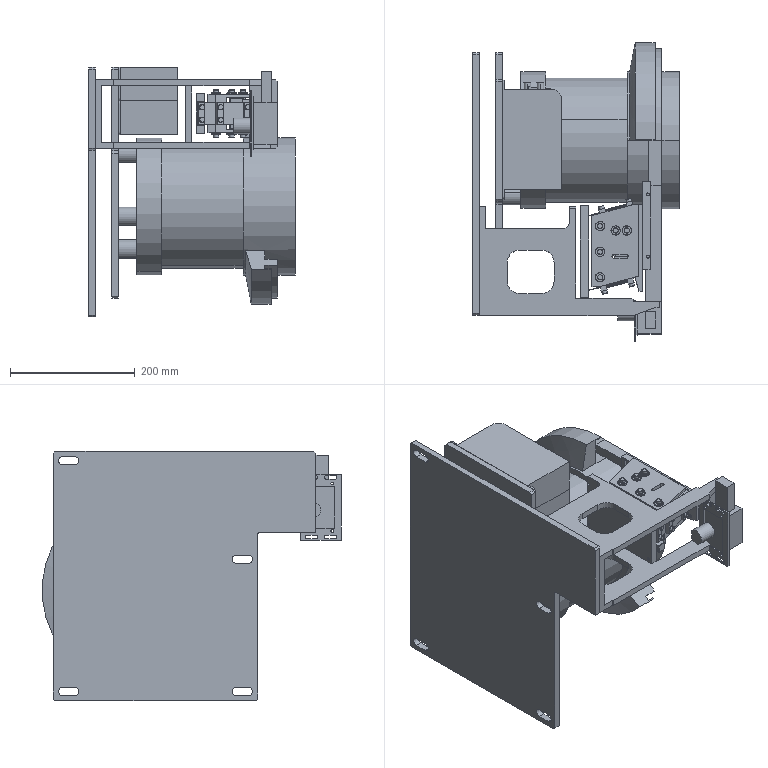Part | STEP file | COMPANY_C blow-air scheme, small part | 14 solids | 1107 faces | box 330.519 x 479.611 x 400.249 mm | volume 15256287 mm3 | plane 618 | cylinder 396 | spline 92 | cone 1 | commonest cylinder face diameters 4.3 x66 8.5 x44 6 x36 5.3 x24 1.289 x20 1.524 x20